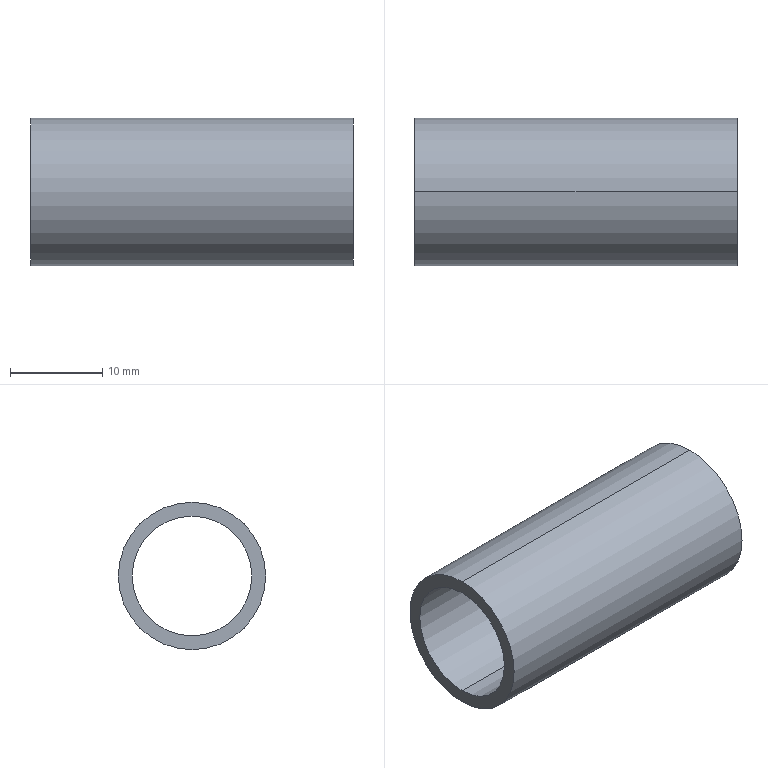Part | STEP file | copper tube 9_default_machined_ | 1 solid | 6 faces | box 35 x 16 x 16 mm | volume 2392 mm3 | cylinder 4 | plane 2 | commonest cylinder face diameters 13 x2 16 x2
STEP:
#1=CARTESIAN_POINT('',(0.,0.,0.));
#2=DIRECTION('',(0.,0.,1.));
#3=DIRECTION('',(1.,0.,0.));
#4=AXIS2_PLACEMENT_3D('',#1,#2,#3);
#5=CARTESIAN_POINT('',(35.,0.,8.));
#6=VERTEX_POINT('',#5);
#7=CARTESIAN_POINT('',(35.,0.,-8.));
#8=VERTEX_POINT('',#7);
#9=CARTESIAN_POINT('',(35.,0.,0.));
#10=DIRECTION('',(-1.,0.,0.));
#11=DIRECTION('',(0.,0.,1.));
#12=AXIS2_PLACEMENT_3D('',#9,#10,#11);
#13=CIRCLE('',#12,8.);
#14=CARTESIAN_POINT('',(35.,0.,0.));
#15=DIRECTION('',(-1.,0.,0.));
#16=DIRECTION('',(0.,0.,1.));
#17=AXIS2_PLACEMENT_3D('',#14,#15,#16);
#18=CYLINDRICAL_SURFACE('',#17,8.);
#19=CARTESIAN_POINT('',(0.,0.));
#20=DIRECTION('',(1.,0.));
#21=VECTOR('',#20,1.);
#22=LINE('',#19,#21);
#23=(GEOMETRIC_REPRESENTATION_CONTEXT(2)PARAMETRIC_REPRESENTATION_CONTEXT()REPRESENTATION_CONTEXT('',''));
#24=DEFINITIONAL_REPRESENTATION('',(#22),#23);
#25=PCURVE('',#18,#24);
#26=CARTESIAN_POINT('',(35.,0.,0.));
#27=DIRECTION('',(1.,0.,0.));
#28=DIRECTION('',(0.,0.,-1.));
#29=AXIS2_PLACEMENT_3D('',#26,#27,#28);
#30=PLANE('',#29);
#31=CARTESIAN_POINT('',(-8.,0.));
#32=CARTESIAN_POINT('',(-8.,13.856));
#33=CARTESIAN_POINT('',(4.,6.928));
#34=CARTESIAN_POINT('',(16.,0.));
#35=CARTESIAN_POINT('',(4.,-6.928));
#36=CARTESIAN_POINT('',(-8.,-13.856));
#37=CARTESIAN_POINT('',(-8.,0.));
#38=(BOUNDED_CURVE()B_SPLINE_CURVE(2,(#31,#32,#33,#34,#35,#36,#37),.UNSPECIFIED.,.T.,.F.)B_SPLINE_CURVE_WITH_KNOTS((1,2,2,2,2,1),(-2.094,0.,2.094,4.189,6.283,8.378),.UNSPECIFIED.)CURVE()GEOMETRIC_REPRESENTATION_ITEM()RATIONAL_B_SPLINE_CURVE((1.,0.5,1.,0.5,1.,0.5,1.))REPRESENTATION_ITEM(''));
#39=(GEOMETRIC_REPRESENTATION_CONTEXT(2)PARAMETRIC_REPRESENTATION_CONTEXT()REPRESENTATION_CONTEXT('',''));
#40=DEFINITIONAL_REPRESENTATION('',(#38),#39);
#41=PCURVE('',#30,#40);
#42=SURFACE_CURVE('',#13,(#25,#41),.PCURVE_S1.);
#43=EDGE_CURVE('',#6,#8,#42,.T.);
#44=ORIENTED_EDGE('',*,*,#43,.T.);
#45=CARTESIAN_POINT('',(0.,0.,-8.));
#46=VERTEX_POINT('',#45);
#47=CARTESIAN_POINT('',(35.,0.,-8.));
#48=DIRECTION('',(-1.,0.,0.));
#49=VECTOR('',#48,1.);
#50=LINE('',#47,#49);
#51=CARTESIAN_POINT('',(3.142,0.));
#52=DIRECTION('',(0.,1.));
#53=VECTOR('',#52,1.);
#54=LINE('',#51,#53);
#55=(GEOMETRIC_REPRESENTATION_CONTEXT(2)PARAMETRIC_REPRESENTATION_CONTEXT()REPRESENTATION_CONTEXT('',''));
#56=DEFINITIONAL_REPRESENTATION('',(#54),#55);
#57=PCURVE('',#18,#56);
#58=CARTESIAN_POINT('',(35.,0.,0.));
#59=DIRECTION('',(-1.,0.,0.));
#60=DIRECTION('',(0.,0.,1.));
#61=AXIS2_PLACEMENT_3D('',#58,#59,#60);
#62=CYLINDRICAL_SURFACE('',#61,8.);
#63=CARTESIAN_POINT('',(3.142,0.));
#64=DIRECTION('',(0.,1.));
#65=VECTOR('',#64,1.);
#66=LINE('',#63,#65);
#67=(GEOMETRIC_REPRESENTATION_CONTEXT(2)PARAMETRIC_REPRESENTATION_CONTEXT()REPRESENTATION_CONTEXT('',''));
#68=DEFINITIONAL_REPRESENTATION('',(#66),#67);
#69=PCURVE('',#62,#68);
#70=SURFACE_CURVE('',#50,(#57,#69),.PCURVE_S1.);
#71=EDGE_CURVE('',#8,#46,#70,.T.);
#72=ORIENTED_EDGE('',*,*,#71,.T.);
#73=CARTESIAN_POINT('',(0.,0.,8.));
#74=VERTEX_POINT('',#73);
#75=CARTESIAN_POINT('',(0.,0.,0.));
#76=DIRECTION('',(1.,0.,0.));
#77=DIRECTION('',(0.,0.,1.));
#78=AXIS2_PLACEMENT_3D('',#75,#76,#77);
#79=CIRCLE('',#78,8.);
#80=CARTESIAN_POINT('',(6.283,35.));
#81=DIRECTION('',(-1.,0.));
#82=VECTOR('',#81,1.);
#83=LINE('',#80,#82);
#84=(GEOMETRIC_REPRESENTATION_CONTEXT(2)PARAMETRIC_REPRESENTATION_CONTEXT()REPRESENTATION_CONTEXT('',''));
#85=DEFINITIONAL_REPRESENTATION('',(#83),#84);
#86=PCURVE('',#18,#85);
#87=CARTESIAN_POINT('',(0.,0.,0.));
#88=DIRECTION('',(1.,0.,0.));
#89=DIRECTION('',(0.,0.,-1.));
#90=AXIS2_PLACEMENT_3D('',#87,#88,#89);
#91=PLANE('',#90);
#92=CARTESIAN_POINT('',(0.,0.));
#93=DIRECTION('',(-1.,0.));
#94=AXIS2_PLACEMENT_2D('',#92,#93);
#95=CIRCLE('',#94,8.);
#96=(GEOMETRIC_REPRESENTATION_CONTEXT(2)PARAMETRIC_REPRESENTATION_CONTEXT()REPRESENTATION_CONTEXT('',''));
#97=DEFINITIONAL_REPRESENTATION('',(#95),#96);
#98=PCURVE('',#91,#97);
#99=SURFACE_CURVE('',#79,(#86,#98),.PCURVE_S1.);
#100=EDGE_CURVE('',#46,#74,#99,.T.);
#101=ORIENTED_EDGE('',*,*,#100,.T.);
#102=CARTESIAN_POINT('',(35.,0.,8.));
#103=DIRECTION('',(-1.,0.,0.));
#104=VECTOR('',#103,1.);
#105=LINE('',#102,#104);
#106=CARTESIAN_POINT('',(0.,0.));
#107=DIRECTION('',(0.,1.));
#108=VECTOR('',#107,1.);
#109=LINE('',#106,#108);
#110=(GEOMETRIC_REPRESENTATION_CONTEXT(2)PARAMETRIC_REPRESENTATION_CONTEXT()REPRESENTATION_CONTEXT('',''));
#111=DEFINITIONAL_REPRESENTATION('',(#109),#110);
#112=PCURVE('',#18,#111);
#113=CARTESIAN_POINT('',(6.283,0.));
#114=DIRECTION('',(0.,1.));
#115=VECTOR('',#114,1.);
#116=LINE('',#113,#115);
#117=(GEOMETRIC_REPRESENTATION_CONTEXT(2)PARAMETRIC_REPRESENTATION_CONTEXT()REPRESENTATION_CONTEXT('',''));
#118=DEFINITIONAL_REPRESENTATION('',(#116),#117);
#119=PCURVE('',#62,#118);
#120=SURFACE_CURVE('',#105,(#112,#119),.PCURVE_S1.);
#121=EDGE_CURVE('',#6,#74,#120,.T.);
#122=ORIENTED_EDGE('',*,*,#121,.F.);
#123=EDGE_LOOP('',(#44,#72,#101,#122));
#124=FACE_BOUND('',#123,.T.);
#125=ADVANCED_FACE('',(#124),#18,.T.);
#126=CARTESIAN_POINT('',(35.,0.,6.5));
#127=VERTEX_POINT('',#126);
#128=CARTESIAN_POINT('',(0.,0.,6.5));
#129=VERTEX_POINT('',#128);
#130=CARTESIAN_POINT('',(35.,0.,6.5));
#131=DIRECTION('',(-1.,0.,0.));
#132=VECTOR('',#131,1.);
#133=LINE('',#130,#132);
#134=CARTESIAN_POINT('',(35.,0.,0.));
#135=DIRECTION('',(-1.,0.,0.));
#136=DIRECTION('',(0.,0.,1.));
#137=AXIS2_PLACEMENT_3D('',#134,#135,#136);
#138=CYLINDRICAL_SURFACE('',#137,6.5);
#139=CARTESIAN_POINT('',(6.283,0.));
#140=DIRECTION('',(0.,1.));
#141=VECTOR('',#140,1.);
#142=LINE('',#139,#141);
#143=(GEOMETRIC_REPRESENTATION_CONTEXT(2)PARAMETRIC_REPRESENTATION_CONTEXT()REPRESENTATION_CONTEXT('',''));
#144=DEFINITIONAL_REPRESENTATION('',(#142),#143);
#145=PCURVE('',#138,#144);
#146=CARTESIAN_POINT('',(35.,0.,0.));
#147=DIRECTION('',(-1.,0.,0.));
#148=DIRECTION('',(0.,0.,1.));
#149=AXIS2_PLACEMENT_3D('',#146,#147,#148);
#150=CYLINDRICAL_SURFACE('',#149,6.5);
#151=CARTESIAN_POINT('',(0.,0.));
#152=DIRECTION('',(0.,1.));
#153=VECTOR('',#152,1.);
#154=LINE('',#151,#153);
#155=(GEOMETRIC_REPRESENTATION_CONTEXT(2)PARAMETRIC_REPRESENTATION_CONTEXT()REPRESENTATION_CONTEXT('',''));
#156=DEFINITIONAL_REPRESENTATION('',(#154),#155);
#157=PCURVE('',#150,#156);
#158=SURFACE_CURVE('',#133,(#145,#157),.PCURVE_S1.);
#159=EDGE_CURVE('',#127,#129,#158,.T.);
#160=ORIENTED_EDGE('',*,*,#159,.T.);
#161=CARTESIAN_POINT('',(0.,0.,-6.5));
#162=VERTEX_POINT('',#161);
#163=CARTESIAN_POINT('',(0.,0.,0.));
#164=DIRECTION('',(-1.,0.,0.));
#165=DIRECTION('',(0.,0.,1.));
#166=AXIS2_PLACEMENT_3D('',#163,#164,#165);
#167=CIRCLE('',#166,6.5);
#168=CARTESIAN_POINT('',(0.,35.));
#169=DIRECTION('',(1.,0.));
#170=VECTOR('',#169,1.);
#171=LINE('',#168,#170);
#172=(GEOMETRIC_REPRESENTATION_CONTEXT(2)PARAMETRIC_REPRESENTATION_CONTEXT()REPRESENTATION_CONTEXT('',''));
#173=DEFINITIONAL_REPRESENTATION('',(#171),#172);
#174=PCURVE('',#138,#173);
#175=CARTESIAN_POINT('',(-6.5,0.));
#176=CARTESIAN_POINT('',(-6.5,11.258));
#177=CARTESIAN_POINT('',(3.25,5.629));
#178=CARTESIAN_POINT('',(13.,0.));
#179=CARTESIAN_POINT('',(3.25,-5.629));
#180=CARTESIAN_POINT('',(-6.5,-11.258));
#181=CARTESIAN_POINT('',(-6.5,0.));
#182=(BOUNDED_CURVE()B_SPLINE_CURVE(2,(#175,#176,#177,#178,#179,#180,#181),.UNSPECIFIED.,.T.,.F.)B_SPLINE_CURVE_WITH_KNOTS((1,2,2,2,2,1),(-2.094,0.,2.094,4.189,6.283,8.378),.UNSPECIFIED.)CURVE()GEOMETRIC_REPRESENTATION_ITEM()RATIONAL_B_SPLINE_CURVE((1.,0.5,1.,0.5,1.,0.5,1.))REPRESENTATION_ITEM(''));
#183=(GEOMETRIC_REPRESENTATION_CONTEXT(2)PARAMETRIC_REPRESENTATION_CONTEXT()REPRESENTATION_CONTEXT('',''));
#184=DEFINITIONAL_REPRESENTATION('',(#182),#183);
#185=PCURVE('',#91,#184);
#186=SURFACE_CURVE('',#167,(#174,#185),.PCURVE_S1.);
#187=EDGE_CURVE('',#162,#129,#186,.T.);
#188=ORIENTED_EDGE('',*,*,#187,.F.);
#189=CARTESIAN_POINT('',(35.,0.,-6.5));
#190=VERTEX_POINT('',#189);
#191=CARTESIAN_POINT('',(35.,0.,-6.5));
#192=DIRECTION('',(-1.,0.,0.));
#193=VECTOR('',#192,1.);
#194=LINE('',#191,#193);
#195=CARTESIAN_POINT('',(3.142,0.));
#196=DIRECTION('',(0.,1.));
#197=VECTOR('',#196,1.);
#198=LINE('',#195,#197);
#199=(GEOMETRIC_REPRESENTATION_CONTEXT(2)PARAMETRIC_REPRESENTATION_CONTEXT()REPRESENTATION_CONTEXT('',''));
#200=DEFINITIONAL_REPRESENTATION('',(#198),#199);
#201=PCURVE('',#138,#200);
#202=CARTESIAN_POINT('',(3.142,0.));
#203=DIRECTION('',(0.,1.));
#204=VECTOR('',#203,1.);
#205=LINE('',#202,#204);
#206=(GEOMETRIC_REPRESENTATION_CONTEXT(2)PARAMETRIC_REPRESENTATION_CONTEXT()REPRESENTATION_CONTEXT('',''));
#207=DEFINITIONAL_REPRESENTATION('',(#205),#206);
#208=PCURVE('',#150,#207);
#209=SURFACE_CURVE('',#194,(#201,#208),.PCURVE_S1.);
#210=EDGE_CURVE('',#190,#162,#209,.T.);
#211=ORIENTED_EDGE('',*,*,#210,.F.);
#212=CARTESIAN_POINT('',(35.,0.,0.));
#213=DIRECTION('',(-1.,0.,0.));
#214=DIRECTION('',(0.,0.,1.));
#215=AXIS2_PLACEMENT_3D('',#212,#213,#214);
#216=CIRCLE('',#215,6.5);
#217=CARTESIAN_POINT('',(0.,0.));
#218=DIRECTION('',(1.,0.));
#219=VECTOR('',#218,1.);
#220=LINE('',#217,#219);
#221=(GEOMETRIC_REPRESENTATION_CONTEXT(2)PARAMETRIC_REPRESENTATION_CONTEXT()REPRESENTATION_CONTEXT('',''));
#222=DEFINITIONAL_REPRESENTATION('',(#220),#221);
#223=PCURVE('',#138,#222);
#224=CARTESIAN_POINT('',(-6.5,0.));
#225=CARTESIAN_POINT('',(-6.5,11.258));
#226=CARTESIAN_POINT('',(3.25,5.629));
#227=CARTESIAN_POINT('',(13.,0.));
#228=CARTESIAN_POINT('',(3.25,-5.629));
#229=CARTESIAN_POINT('',(-6.5,-11.258));
#230=CARTESIAN_POINT('',(-6.5,0.));
#231=(BOUNDED_CURVE()B_SPLINE_CURVE(2,(#224,#225,#226,#227,#228,#229,#230),.UNSPECIFIED.,.T.,.F.)B_SPLINE_CURVE_WITH_KNOTS((1,2,2,2,2,1),(-2.094,0.,2.094,4.189,6.283,8.378),.UNSPECIFIED.)CURVE()GEOMETRIC_REPRESENTATION_ITEM()RATIONAL_B_SPLINE_CURVE((1.,0.5,1.,0.5,1.,0.5,1.))REPRESENTATION_ITEM(''));
#232=(GEOMETRIC_REPRESENTATION_CONTEXT(2)PARAMETRIC_REPRESENTATION_CONTEXT()REPRESENTATION_CONTEXT('',''));
#233=DEFINITIONAL_REPRESENTATION('',(#231),#232);
#234=PCURVE('',#30,#233);
#235=SURFACE_CURVE('',#216,(#223,#234),.PCURVE_S1.);
#236=EDGE_CURVE('',#190,#127,#235,.T.);
#237=ORIENTED_EDGE('',*,*,#236,.T.);
#238=EDGE_LOOP('',(#160,#188,#211,#237));
#239=FACE_BOUND('',#238,.F.);
#240=ADVANCED_FACE('',(#239),#138,.F.);
#241=ORIENTED_EDGE('',*,*,#71,.F.);
#242=CARTESIAN_POINT('',(35.,0.,0.));
#243=DIRECTION('',(-1.,0.,0.));
#244=DIRECTION('',(0.,0.,1.));
#245=AXIS2_PLACEMENT_3D('',#242,#243,#244);
#246=CIRCLE('',#245,8.);
#247=CARTESIAN_POINT('',(0.,0.));
#248=DIRECTION('',(1.,0.));
#249=VECTOR('',#248,1.);
#250=LINE('',#247,#249);
#251=(GEOMETRIC_REPRESENTATION_CONTEXT(2)PARAMETRIC_REPRESENTATION_CONTEXT()REPRESENTATION_CONTEXT('',''));
#252=DEFINITIONAL_REPRESENTATION('',(#250),#251);
#253=PCURVE('',#62,#252);
#254=CARTESIAN_POINT('',(-8.,0.));
#255=CARTESIAN_POINT('',(-8.,13.856));
#256=CARTESIAN_POINT('',(4.,6.928));
#257=CARTESIAN_POINT('',(16.,0.));
#258=CARTESIAN_POINT('',(4.,-6.928));
#259=CARTESIAN_POINT('',(-8.,-13.856));
#260=CARTESIAN_POINT('',(-8.,0.));
#261=(BOUNDED_CURVE()B_SPLINE_CURVE(2,(#254,#255,#256,#257,#258,#259,#260),.UNSPECIFIED.,.T.,.F.)B_SPLINE_CURVE_WITH_KNOTS((1,2,2,2,2,1),(-2.094,0.,2.094,4.189,6.283,8.378),.UNSPECIFIED.)CURVE()GEOMETRIC_REPRESENTATION_ITEM()RATIONAL_B_SPLINE_CURVE((1.,0.5,1.,0.5,1.,0.5,1.))REPRESENTATION_ITEM(''));
#262=(GEOMETRIC_REPRESENTATION_CONTEXT(2)PARAMETRIC_REPRESENTATION_CONTEXT()REPRESENTATION_CONTEXT('',''));
#263=DEFINITIONAL_REPRESENTATION('',(#261),#262);
#264=PCURVE('',#30,#263);
#265=SURFACE_CURVE('',#246,(#253,#264),.PCURVE_S1.);
#266=EDGE_CURVE('',#8,#6,#265,.T.);
#267=ORIENTED_EDGE('',*,*,#266,.T.);
#268=ORIENTED_EDGE('',*,*,#121,.T.);
#269=CARTESIAN_POINT('',(0.,0.,0.));
#270=DIRECTION('',(1.,0.,0.));
#271=DIRECTION('',(0.,0.,1.));
#272=AXIS2_PLACEMENT_3D('',#269,#270,#271);
#273=CIRCLE('',#272,8.);
#274=CARTESIAN_POINT('',(6.283,35.));
#275=DIRECTION('',(-1.,0.));
#276=VECTOR('',#275,1.);
#277=LINE('',#274,#276);
#278=(GEOMETRIC_REPRESENTATION_CONTEXT(2)PARAMETRIC_REPRESENTATION_CONTEXT()REPRESENTATION_CONTEXT('',''));
#279=DEFINITIONAL_REPRESENTATION('',(#277),#278);
#280=PCURVE('',#62,#279);
#281=CARTESIAN_POINT('',(0.,0.));
#282=DIRECTION('',(-1.,0.));
#283=AXIS2_PLACEMENT_2D('',#281,#282);
#284=CIRCLE('',#283,8.);
#285=(GEOMETRIC_REPRESENTATION_CONTEXT(2)PARAMETRIC_REPRESENTATION_CONTEXT()REPRESENTATION_CONTEXT('',''));
#286=DEFINITIONAL_REPRESENTATION('',(#284),#285);
#287=PCURVE('',#91,#286);
#288=SURFACE_CURVE('',#273,(#280,#287),.PCURVE_S1.);
#289=EDGE_CURVE('',#74,#46,#288,.T.);
#290=ORIENTED_EDGE('',*,*,#289,.T.);
#291=EDGE_LOOP('',(#241,#267,#268,#290));
#292=FACE_BOUND('',#291,.T.);
#293=ADVANCED_FACE('',(#292),#62,.T.);
#294=ORIENTED_EDGE('',*,*,#289,.F.);
#295=ORIENTED_EDGE('',*,*,#100,.F.);
#296=EDGE_LOOP('',(#294,#295));
#297=FACE_BOUND('',#296,.T.);
#298=CARTESIAN_POINT('',(0.,0.,0.));
#299=DIRECTION('',(-1.,0.,0.));
#300=DIRECTION('',(0.,0.,1.));
#301=AXIS2_PLACEMENT_3D('',#298,#299,#300);
#302=CIRCLE('',#301,6.5);
#303=CARTESIAN_POINT('',(-6.5,0.));
#304=CARTESIAN_POINT('',(-6.5,11.258));
#305=CARTESIAN_POINT('',(3.25,5.629));
#306=CARTESIAN_POINT('',(13.,0.));
#307=CARTESIAN_POINT('',(3.25,-5.629));
#308=CARTESIAN_POINT('',(-6.5,-11.258));
#309=CARTESIAN_POINT('',(-6.5,0.));
#310=(BOUNDED_CURVE()B_SPLINE_CURVE(2,(#303,#304,#305,#306,#307,#308,#309),.UNSPECIFIED.,.T.,.F.)B_SPLINE_CURVE_WITH_KNOTS((1,2,2,2,2,1),(-2.094,0.,2.094,4.189,6.283,8.378),.UNSPECIFIED.)CURVE()GEOMETRIC_REPRESENTATION_ITEM()RATIONAL_B_SPLINE_CURVE((1.,0.5,1.,0.5,1.,0.5,1.))REPRESENTATION_ITEM(''));
#311=(GEOMETRIC_REPRESENTATION_CONTEXT(2)PARAMETRIC_REPRESENTATION_CONTEXT()REPRESENTATION_CONTEXT('',''));
#312=DEFINITIONAL_REPRESENTATION('',(#310),#311);
#313=PCURVE('',#91,#312);
#314=CARTESIAN_POINT('',(0.,35.));
#315=DIRECTION('',(1.,0.));
#316=VECTOR('',#315,1.);
#317=LINE('',#314,#316);
#318=(GEOMETRIC_REPRESENTATION_CONTEXT(2)PARAMETRIC_REPRESENTATION_CONTEXT()REPRESENTATION_CONTEXT('',''));
#319=DEFINITIONAL_REPRESENTATION('',(#317),#318);
#320=PCURVE('',#150,#319);
#321=SURFACE_CURVE('',#302,(#313,#320),.PCURVE_S1.);
#322=EDGE_CURVE('',#129,#162,#321,.T.);
#323=ORIENTED_EDGE('',*,*,#322,.F.);
#324=ORIENTED_EDGE('',*,*,#187,.F.);
#325=EDGE_LOOP('',(#323,#324));
#326=FACE_BOUND('',#325,.T.);
#327=ADVANCED_FACE('',(#297,#326),#91,.F.);
#328=ORIENTED_EDGE('',*,*,#43,.F.);
#329=ORIENTED_EDGE('',*,*,#266,.F.);
#330=EDGE_LOOP('',(#328,#329));
#331=FACE_BOUND('',#330,.T.);
#332=CARTESIAN_POINT('',(35.,0.,0.));
#333=DIRECTION('',(-1.,0.,0.));
#334=DIRECTION('',(0.,0.,1.));
#335=AXIS2_PLACEMENT_3D('',#332,#333,#334);
#336=CIRCLE('',#335,6.5);
#337=CARTESIAN_POINT('',(-6.5,0.));
#338=CARTESIAN_POINT('',(-6.5,11.258));
#339=CARTESIAN_POINT('',(3.25,5.629));
#340=CARTESIAN_POINT('',(13.,0.));
#341=CARTESIAN_POINT('',(3.25,-5.629));
#342=CARTESIAN_POINT('',(-6.5,-11.258));
#343=CARTESIAN_POINT('',(-6.5,0.));
#344=(BOUNDED_CURVE()B_SPLINE_CURVE(2,(#337,#338,#339,#340,#341,#342,#343),.UNSPECIFIED.,.T.,.F.)B_SPLINE_CURVE_WITH_KNOTS((1,2,2,2,2,1),(-2.094,0.,2.094,4.189,6.283,8.378),.UNSPECIFIED.)CURVE()GEOMETRIC_REPRESENTATION_ITEM()RATIONAL_B_SPLINE_CURVE((1.,0.5,1.,0.5,1.,0.5,1.))REPRESENTATION_ITEM(''));
#345=(GEOMETRIC_REPRESENTATION_CONTEXT(2)PARAMETRIC_REPRESENTATION_CONTEXT()REPRESENTATION_CONTEXT('',''));
#346=DEFINITIONAL_REPRESENTATION('',(#344),#345);
#347=PCURVE('',#30,#346);
#348=CARTESIAN_POINT('',(0.,0.));
#349=DIRECTION('',(1.,0.));
#350=VECTOR('',#349,1.);
#351=LINE('',#348,#350);
#352=(GEOMETRIC_REPRESENTATION_CONTEXT(2)PARAMETRIC_REPRESENTATION_CONTEXT()REPRESENTATION_CONTEXT('',''));
#353=DEFINITIONAL_REPRESENTATION('',(#351),#352);
#354=PCURVE('',#150,#353);
#355=SURFACE_CURVE('',#336,(#347,#354),.PCURVE_S1.);
#356=EDGE_CURVE('',#127,#190,#355,.T.);
#357=ORIENTED_EDGE('',*,*,#356,.T.);
#358=ORIENTED_EDGE('',*,*,#236,.T.);
#359=EDGE_LOOP('',(#357,#358));
#360=FACE_BOUND('',#359,.T.);
#361=ADVANCED_FACE('',(#331,#360),#30,.T.);
#362=ORIENTED_EDGE('',*,*,#322,.F.);
#363=ORIENTED_EDGE('',*,*,#159,.F.);
#364=ORIENTED_EDGE('',*,*,#356,.T.);
#365=ORIENTED_EDGE('',*,*,#210,.T.);
#366=EDGE_LOOP('',(#362,#363,#364,#365));
#367=FACE_BOUND('',#366,.F.);
#368=ADVANCED_FACE('',(#367),#150,.F.);
#369=CLOSED_SHELL('',(#125,#240,#293,#327,#361,#368));
#370=MANIFOLD_SOLID_BREP('',#369);
#371=(LENGTH_UNIT()NAMED_UNIT(*)SI_UNIT(.MILLI.,.METRE.));
#372=UNCERTAINTY_MEASURE_WITH_UNIT(LENGTH_MEASURE(0.0000001),#371,'','');
#373=(NAMED_UNIT(*)PLANE_ANGLE_UNIT()SI_UNIT($,.RADIAN.));
#374=(NAMED_UNIT(*)SI_UNIT($,.STERADIAN.)SOLID_ANGLE_UNIT());
#375=(GEOMETRIC_REPRESENTATION_CONTEXT(3)GLOBAL_UNCERTAINTY_ASSIGNED_CONTEXT((#372))GLOBAL_UNIT_ASSIGNED_CONTEXT((#371,#373,#374))REPRESENTATION_CONTEXT('',''));
#376=ADVANCED_BREP_SHAPE_REPRESENTATION('',(#4,#370),#375);